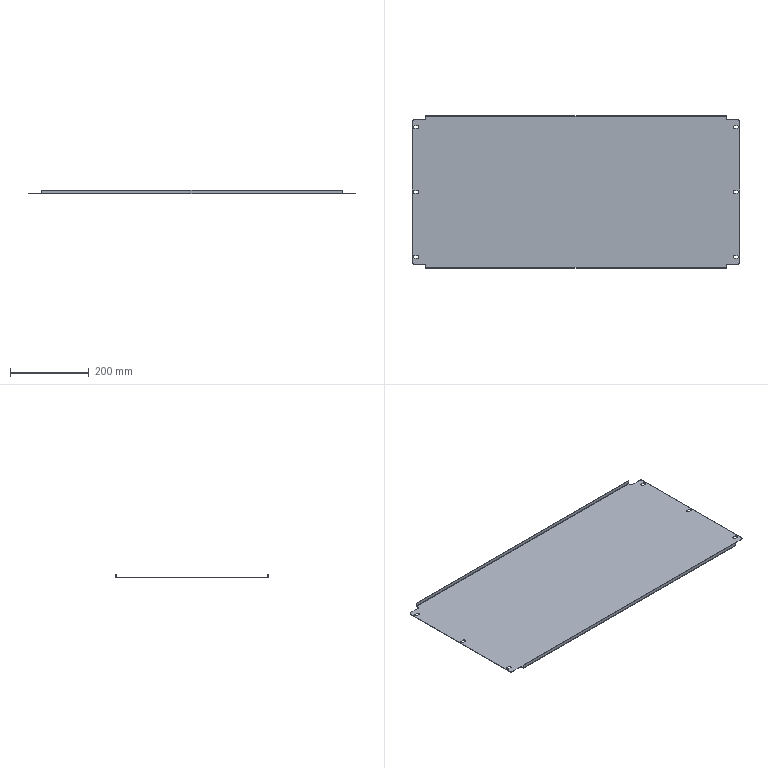Part | SolidWorks | features ICE 3, EdgeFlange 1, Fillet 1, FlatPattern 1, SMBaseFlange 1, SheetMetal 1 | 1 solid | 68 faces | box 830 x 385 x 10 mm | volume 330695 mm3 | plane 38 | cylinder 30 | commonest cylinder face diameters 7 x18 10 x8 1 x2 3 x2